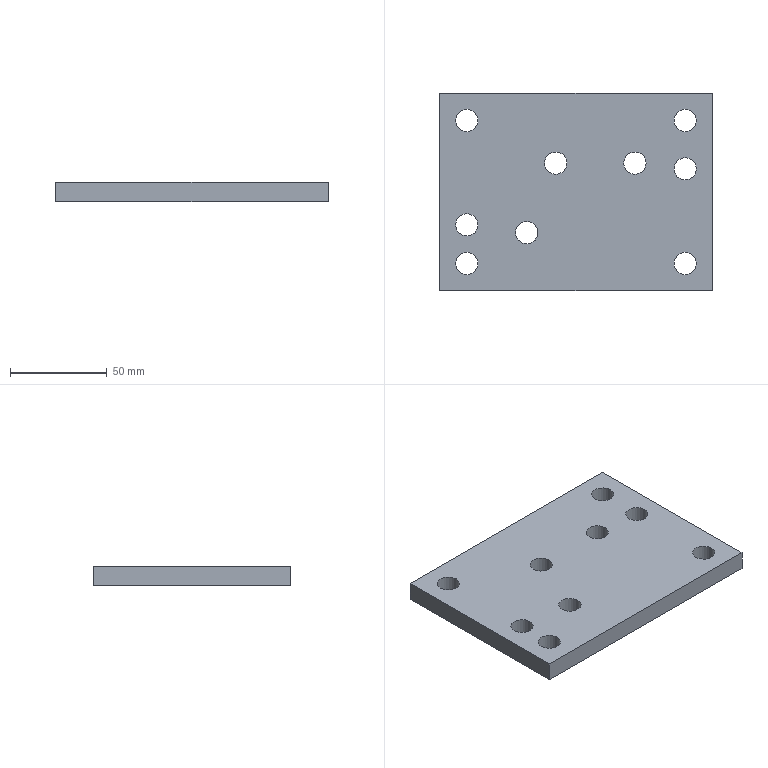Part | NX | features 6 2 | 1 solid | 15 faces | box 141 x 102 x 10 mm | volume 134472 mm3 | cylinder 9 | plane 6 | commonest cylinder face diameters 11.5 x9
STEP:
#1=CARTESIAN_POINT('',(177.279,-375.95,91.));
#2=VERTEX_POINT('',#1);
#3=CARTESIAN_POINT('',(171.529,-375.95,91.));
#4=DIRECTION('',(0.,0.,1.));
#5=DIRECTION('',(1.,0.,0.));
#6=AXIS2_PLACEMENT_3D('',#3,#4,#5);
#7=CIRCLE('',#6,5.75);
#8=EDGE_CURVE('',#2,#2,#7,.T.);
#9=ORIENTED_EDGE('',*,*,#8,.F.);
#10=EDGE_LOOP('',(#9));
#11=FACE_BOUND('',#10,.T.);
#12=CARTESIAN_POINT('',(177.279,-375.95,101.));
#13=VERTEX_POINT('',#12);
#14=CARTESIAN_POINT('',(171.529,-375.95,101.));
#15=DIRECTION('',(0.,0.,1.));
#16=DIRECTION('',(1.,0.,0.));
#17=AXIS2_PLACEMENT_3D('',#14,#15,#16);
#18=CIRCLE('',#17,5.75);
#19=EDGE_CURVE('',#13,#13,#18,.T.);
#20=ORIENTED_EDGE('',*,*,#19,.T.);
#21=EDGE_LOOP('',(#20));
#22=FACE_BOUND('',#21,.T.);
#23=CARTESIAN_POINT('',(171.529,-375.95,91.));
#24=DIRECTION('',(0.,0.,1.));
#25=DIRECTION('',(-1.,0.,0.));
#26=AXIS2_PLACEMENT_3D('',#23,#24,#25);
#27=CYLINDRICAL_SURFACE('',#26,5.75);
#28=ADVANCED_FACE('',(#11,#22),#27,.F.);
#29=CARTESIAN_POINT('',(64.279,-429.95,91.));
#30=VERTEX_POINT('',#29);
#31=CARTESIAN_POINT('',(58.529,-429.95,91.));
#32=DIRECTION('',(0.,0.,1.));
#33=DIRECTION('',(1.,0.,0.));
#34=AXIS2_PLACEMENT_3D('',#31,#32,#33);
#35=CIRCLE('',#34,5.75);
#36=EDGE_CURVE('',#30,#30,#35,.T.);
#37=ORIENTED_EDGE('',*,*,#36,.F.);
#38=EDGE_LOOP('',(#37));
#39=FACE_BOUND('',#38,.T.);
#40=CARTESIAN_POINT('',(64.279,-429.95,101.));
#41=VERTEX_POINT('',#40);
#42=CARTESIAN_POINT('',(58.529,-429.95,101.));
#43=DIRECTION('',(0.,0.,-1.));
#44=DIRECTION('',(1.,0.,0.));
#45=AXIS2_PLACEMENT_3D('',#42,#43,#44);
#46=CIRCLE('',#45,5.75);
#47=EDGE_CURVE('',#41,#41,#46,.T.);
#48=ORIENTED_EDGE('',*,*,#47,.F.);
#49=EDGE_LOOP('',(#48));
#50=FACE_BOUND('',#49,.T.);
#51=CARTESIAN_POINT('',(58.529,-429.95,91.));
#52=DIRECTION('',(0.,0.,1.));
#53=DIRECTION('',(-1.,0.,0.));
#54=AXIS2_PLACEMENT_3D('',#51,#52,#53);
#55=CYLINDRICAL_SURFACE('',#54,5.75);
#56=ADVANCED_FACE('',(#39,#50),#55,.F.);
#57=CARTESIAN_POINT('',(64.279,-375.95,91.));
#58=VERTEX_POINT('',#57);
#59=CARTESIAN_POINT('',(58.529,-375.95,91.));
#60=DIRECTION('',(0.,0.,-1.));
#61=DIRECTION('',(1.,0.,0.));
#62=AXIS2_PLACEMENT_3D('',#59,#60,#61);
#63=CIRCLE('',#62,5.75);
#64=EDGE_CURVE('',#58,#58,#63,.T.);
#65=ORIENTED_EDGE('',*,*,#64,.T.);
#66=EDGE_LOOP('',(#65));
#67=FACE_BOUND('',#66,.T.);
#68=CARTESIAN_POINT('',(64.279,-375.95,101.));
#69=VERTEX_POINT('',#68);
#70=CARTESIAN_POINT('',(58.529,-375.95,101.));
#71=DIRECTION('',(0.,0.,-1.));
#72=DIRECTION('',(1.,0.,0.));
#73=AXIS2_PLACEMENT_3D('',#70,#71,#72);
#74=CIRCLE('',#73,5.75);
#75=EDGE_CURVE('',#69,#69,#74,.T.);
#76=ORIENTED_EDGE('',*,*,#75,.F.);
#77=EDGE_LOOP('',(#76));
#78=FACE_BOUND('',#77,.T.);
#79=CARTESIAN_POINT('',(58.529,-375.95,91.));
#80=DIRECTION('',(0.,0.,1.));
#81=DIRECTION('',(-1.,0.,0.));
#82=AXIS2_PLACEMENT_3D('',#79,#80,#81);
#83=CYLINDRICAL_SURFACE('',#82,5.75);
#84=ADVANCED_FACE('',(#67,#78),#83,.F.);
#85=CARTESIAN_POINT('',(185.529,-463.95,91.));
#86=VERTEX_POINT('',#85);
#87=CARTESIAN_POINT('',(185.529,-463.95,101.));
#88=VERTEX_POINT('',#87);
#89=CARTESIAN_POINT('',(185.529,-463.95,91.));
#90=DIRECTION('',(0.,0.,1.));
#91=VECTOR('',#90,1000.);
#92=LINE('',#89,#91);
#93=EDGE_CURVE('',#86,#88,#92,.T.);
#94=ORIENTED_EDGE('',*,*,#93,.F.);
#95=CARTESIAN_POINT('',(185.529,-361.95,91.));
#96=VERTEX_POINT('',#95);
#97=CARTESIAN_POINT('',(185.529,-411.95,91.));
#98=DIRECTION('',(0.,1.,0.));
#99=VECTOR('',#98,1000.);
#100=LINE('',#97,#99);
#101=EDGE_CURVE('',#86,#96,#100,.T.);
#102=ORIENTED_EDGE('',*,*,#101,.T.);
#103=CARTESIAN_POINT('',(185.529,-361.95,101.));
#104=VERTEX_POINT('',#103);
#105=CARTESIAN_POINT('',(185.529,-361.95,91.));
#106=DIRECTION('',(0.,0.,1.));
#107=VECTOR('',#106,1000.);
#108=LINE('',#105,#107);
#109=EDGE_CURVE('',#96,#104,#108,.T.);
#110=ORIENTED_EDGE('',*,*,#109,.T.);
#111=CARTESIAN_POINT('',(185.529,-411.95,101.));
#112=DIRECTION('',(0.,1.,0.));
#113=VECTOR('',#112,1000.);
#114=LINE('',#111,#113);
#115=EDGE_CURVE('',#88,#104,#114,.T.);
#116=ORIENTED_EDGE('',*,*,#115,.F.);
#117=EDGE_LOOP('',(#94,#102,#110,#116));
#118=FACE_BOUND('',#117,.T.);
#119=CARTESIAN_POINT('',(185.529,-411.95,91.));
#120=DIRECTION('',(-1.,0.,0.));
#121=DIRECTION('',(0.,1.,0.));
#122=AXIS2_PLACEMENT_3D('',#119,#120,#121);
#123=PLANE('',#122);
#124=ADVANCED_FACE('',(#118),#123,.F.);
#125=ORIENTED_EDGE('',*,*,#109,.F.);
#126=CARTESIAN_POINT('',(44.529,-361.95,91.));
#127=VERTEX_POINT('',#126);
#128=CARTESIAN_POINT('',(87.029,-361.95,91.));
#129=DIRECTION('',(-1.,0.,0.));
#130=VECTOR('',#129,1000.);
#131=LINE('',#128,#130);
#132=EDGE_CURVE('',#96,#127,#131,.T.);
#133=ORIENTED_EDGE('',*,*,#132,.T.);
#134=CARTESIAN_POINT('',(44.529,-361.95,101.));
#135=VERTEX_POINT('',#134);
#136=CARTESIAN_POINT('',(44.529,-361.95,91.));
#137=DIRECTION('',(0.,0.,1.));
#138=VECTOR('',#137,1000.);
#139=LINE('',#136,#138);
#140=EDGE_CURVE('',#127,#135,#139,.T.);
#141=ORIENTED_EDGE('',*,*,#140,.T.);
#142=CARTESIAN_POINT('',(87.029,-361.95,101.));
#143=DIRECTION('',(-1.,0.,0.));
#144=VECTOR('',#143,1000.);
#145=LINE('',#142,#144);
#146=EDGE_CURVE('',#104,#135,#145,.T.);
#147=ORIENTED_EDGE('',*,*,#146,.F.);
#148=EDGE_LOOP('',(#125,#133,#141,#147));
#149=FACE_BOUND('',#148,.T.);
#150=CARTESIAN_POINT('',(87.029,-361.95,91.));
#151=DIRECTION('',(0.,-1.,0.));
#152=DIRECTION('',(-1.,0.,0.));
#153=AXIS2_PLACEMENT_3D('',#150,#151,#152);
#154=PLANE('',#153);
#155=ADVANCED_FACE('',(#149),#154,.F.);
#156=ORIENTED_EDGE('',*,*,#140,.F.);
#157=CARTESIAN_POINT('',(44.529,-463.95,91.));
#158=VERTEX_POINT('',#157);
#159=CARTESIAN_POINT('',(44.529,-411.95,91.));
#160=DIRECTION('',(0.,-1.,0.));
#161=VECTOR('',#160,1000.);
#162=LINE('',#159,#161);
#163=EDGE_CURVE('',#127,#158,#162,.T.);
#164=ORIENTED_EDGE('',*,*,#163,.T.);
#165=CARTESIAN_POINT('',(44.529,-463.95,101.));
#166=VERTEX_POINT('',#165);
#167=CARTESIAN_POINT('',(44.529,-463.95,91.));
#168=DIRECTION('',(0.,0.,1.));
#169=VECTOR('',#168,1000.);
#170=LINE('',#167,#169);
#171=EDGE_CURVE('',#158,#166,#170,.T.);
#172=ORIENTED_EDGE('',*,*,#171,.T.);
#173=CARTESIAN_POINT('',(44.529,-411.95,101.));
#174=DIRECTION('',(0.,-1.,0.));
#175=VECTOR('',#174,1000.);
#176=LINE('',#173,#175);
#177=EDGE_CURVE('',#135,#166,#176,.T.);
#178=ORIENTED_EDGE('',*,*,#177,.F.);
#179=EDGE_LOOP('',(#156,#164,#172,#178));
#180=FACE_BOUND('',#179,.T.);
#181=CARTESIAN_POINT('',(44.529,-411.95,91.));
#182=DIRECTION('',(1.,0.,0.));
#183=DIRECTION('',(0.,-1.,0.));
#184=AXIS2_PLACEMENT_3D('',#181,#182,#183);
#185=PLANE('',#184);
#186=ADVANCED_FACE('',(#180),#185,.F.);
#187=ORIENTED_EDGE('',*,*,#171,.F.);
#188=CARTESIAN_POINT('',(87.029,-463.95,91.));
#189=DIRECTION('',(1.,0.,0.));
#190=VECTOR('',#189,1000.);
#191=LINE('',#188,#190);
#192=EDGE_CURVE('',#158,#86,#191,.T.);
#193=ORIENTED_EDGE('',*,*,#192,.T.);
#194=ORIENTED_EDGE('',*,*,#93,.T.);
#195=CARTESIAN_POINT('',(87.029,-463.95,101.));
#196=DIRECTION('',(1.,0.,0.));
#197=VECTOR('',#196,1000.);
#198=LINE('',#195,#197);
#199=EDGE_CURVE('',#166,#88,#198,.T.);
#200=ORIENTED_EDGE('',*,*,#199,.F.);
#201=EDGE_LOOP('',(#187,#193,#194,#200));
#202=FACE_BOUND('',#201,.T.);
#203=CARTESIAN_POINT('',(87.029,-463.95,91.));
#204=DIRECTION('',(0.,1.,0.));
#205=DIRECTION('',(1.,0.,0.));
#206=AXIS2_PLACEMENT_3D('',#203,#204,#205);
#207=PLANE('',#206);
#208=ADVANCED_FACE('',(#202),#207,.F.);
#209=CARTESIAN_POINT('',(177.279,-449.95,91.));
#210=VERTEX_POINT('',#209);
#211=CARTESIAN_POINT('',(171.529,-449.95,91.));
#212=DIRECTION('',(0.,0.,-1.));
#213=DIRECTION('',(1.,0.,0.));
#214=AXIS2_PLACEMENT_3D('',#211,#212,#213);
#215=CIRCLE('',#214,5.75);
#216=EDGE_CURVE('',#210,#210,#215,.T.);
#217=ORIENTED_EDGE('',*,*,#216,.T.);
#218=EDGE_LOOP('',(#217));
#219=FACE_BOUND('',#218,.T.);
#220=CARTESIAN_POINT('',(177.279,-449.95,101.));
#221=VERTEX_POINT('',#220);
#222=CARTESIAN_POINT('',(171.529,-449.95,101.));
#223=DIRECTION('',(0.,0.,-1.));
#224=DIRECTION('',(1.,0.,0.));
#225=AXIS2_PLACEMENT_3D('',#222,#223,#224);
#226=CIRCLE('',#225,5.75);
#227=EDGE_CURVE('',#221,#221,#226,.T.);
#228=ORIENTED_EDGE('',*,*,#227,.F.);
#229=EDGE_LOOP('',(#228));
#230=FACE_BOUND('',#229,.T.);
#231=CARTESIAN_POINT('',(171.529,-449.95,91.));
#232=DIRECTION('',(0.,0.,1.));
#233=DIRECTION('',(-1.,0.,0.));
#234=AXIS2_PLACEMENT_3D('',#231,#232,#233);
#235=CYLINDRICAL_SURFACE('',#234,5.75);
#236=ADVANCED_FACE('',(#219,#230),#235,.F.);
#237=CARTESIAN_POINT('',(177.279,-400.95,91.));
#238=VERTEX_POINT('',#237);
#239=CARTESIAN_POINT('',(171.529,-400.95,91.));
#240=DIRECTION('',(0.,0.,1.));
#241=DIRECTION('',(1.,0.,0.));
#242=AXIS2_PLACEMENT_3D('',#239,#240,#241);
#243=CIRCLE('',#242,5.75);
#244=EDGE_CURVE('',#238,#238,#243,.T.);
#245=ORIENTED_EDGE('',*,*,#244,.F.);
#246=EDGE_LOOP('',(#245));
#247=FACE_BOUND('',#246,.T.);
#248=CARTESIAN_POINT('',(177.279,-400.95,101.));
#249=VERTEX_POINT('',#248);
#250=CARTESIAN_POINT('',(171.529,-400.95,101.));
#251=DIRECTION('',(0.,0.,-1.));
#252=DIRECTION('',(1.,0.,0.));
#253=AXIS2_PLACEMENT_3D('',#250,#251,#252);
#254=CIRCLE('',#253,5.75);
#255=EDGE_CURVE('',#249,#249,#254,.T.);
#256=ORIENTED_EDGE('',*,*,#255,.F.);
#257=EDGE_LOOP('',(#256));
#258=FACE_BOUND('',#257,.T.);
#259=CARTESIAN_POINT('',(171.529,-400.95,91.));
#260=DIRECTION('',(0.,0.,1.));
#261=DIRECTION('',(-1.,0.,0.));
#262=AXIS2_PLACEMENT_3D('',#259,#260,#261);
#263=CYLINDRICAL_SURFACE('',#262,5.75);
#264=ADVANCED_FACE('',(#247,#258),#263,.F.);
#265=CARTESIAN_POINT('',(64.279,-449.95,91.));
#266=VERTEX_POINT('',#265);
#267=CARTESIAN_POINT('',(58.529,-449.95,91.));
#268=DIRECTION('',(0.,0.,1.));
#269=DIRECTION('',(1.,0.,0.));
#270=AXIS2_PLACEMENT_3D('',#267,#268,#269);
#271=CIRCLE('',#270,5.75);
#272=EDGE_CURVE('',#266,#266,#271,.T.);
#273=ORIENTED_EDGE('',*,*,#272,.F.);
#274=EDGE_LOOP('',(#273));
#275=FACE_BOUND('',#274,.T.);
#276=CARTESIAN_POINT('',(64.279,-449.95,101.));
#277=VERTEX_POINT('',#276);
#278=CARTESIAN_POINT('',(58.529,-449.95,101.));
#279=DIRECTION('',(0.,0.,1.));
#280=DIRECTION('',(1.,0.,0.));
#281=AXIS2_PLACEMENT_3D('',#278,#279,#280);
#282=CIRCLE('',#281,5.75);
#283=EDGE_CURVE('',#277,#277,#282,.T.);
#284=ORIENTED_EDGE('',*,*,#283,.T.);
#285=EDGE_LOOP('',(#284));
#286=FACE_BOUND('',#285,.T.);
#287=CARTESIAN_POINT('',(58.529,-449.95,91.));
#288=DIRECTION('',(0.,0.,1.));
#289=DIRECTION('',(-1.,0.,0.));
#290=AXIS2_PLACEMENT_3D('',#287,#288,#289);
#291=CYLINDRICAL_SURFACE('',#290,5.75);
#292=ADVANCED_FACE('',(#275,#286),#291,.F.);
#293=CARTESIAN_POINT('',(95.279,-434.,91.));
#294=VERTEX_POINT('',#293);
#295=CARTESIAN_POINT('',(89.529,-434.,91.));
#296=DIRECTION('',(0.,0.,-1.));
#297=DIRECTION('',(1.,0.,0.));
#298=AXIS2_PLACEMENT_3D('',#295,#296,#297);
#299=CIRCLE('',#298,5.75);
#300=EDGE_CURVE('',#294,#294,#299,.T.);
#301=ORIENTED_EDGE('',*,*,#300,.F.);
#302=EDGE_LOOP('',(#301));
#303=FACE_BOUND('',#302,.T.);
#304=CARTESIAN_POINT('',(110.279,-398.,91.));
#305=VERTEX_POINT('',#304);
#306=CARTESIAN_POINT('',(104.529,-398.,91.));
#307=DIRECTION('',(0.,0.,-1.));
#308=DIRECTION('',(1.,0.,0.));
#309=AXIS2_PLACEMENT_3D('',#306,#307,#308);
#310=CIRCLE('',#309,5.75);
#311=EDGE_CURVE('',#305,#305,#310,.T.);
#312=ORIENTED_EDGE('',*,*,#311,.F.);
#313=EDGE_LOOP('',(#312));
#314=FACE_BOUND('',#313,.T.);
#315=CARTESIAN_POINT('',(151.279,-398.,91.));
#316=VERTEX_POINT('',#315);
#317=CARTESIAN_POINT('',(145.529,-398.,91.));
#318=DIRECTION('',(0.,0.,1.));
#319=DIRECTION('',(1.,0.,0.));
#320=AXIS2_PLACEMENT_3D('',#317,#318,#319);
#321=CIRCLE('',#320,5.75);
#322=EDGE_CURVE('',#316,#316,#321,.T.);
#323=ORIENTED_EDGE('',*,*,#322,.T.);
#324=EDGE_LOOP('',(#323));
#325=FACE_BOUND('',#324,.T.);
#326=ORIENTED_EDGE('',*,*,#8,.T.);
#327=EDGE_LOOP('',(#326));
#328=FACE_BOUND('',#327,.T.);
#329=ORIENTED_EDGE('',*,*,#272,.T.);
#330=EDGE_LOOP('',(#329));
#331=FACE_BOUND('',#330,.T.);
#332=ORIENTED_EDGE('',*,*,#244,.T.);
#333=EDGE_LOOP('',(#332));
#334=FACE_BOUND('',#333,.T.);
#335=ORIENTED_EDGE('',*,*,#216,.F.);
#336=EDGE_LOOP('',(#335));
#337=FACE_BOUND('',#336,.T.);
#338=ORIENTED_EDGE('',*,*,#192,.F.);
#339=ORIENTED_EDGE('',*,*,#163,.F.);
#340=ORIENTED_EDGE('',*,*,#132,.F.);
#341=ORIENTED_EDGE('',*,*,#101,.F.);
#342=EDGE_LOOP('',(#338,#339,#340,#341));
#343=FACE_BOUND('',#342,.T.);
#344=ORIENTED_EDGE('',*,*,#64,.F.);
#345=EDGE_LOOP('',(#344));
#346=FACE_BOUND('',#345,.T.);
#347=ORIENTED_EDGE('',*,*,#36,.T.);
#348=EDGE_LOOP('',(#347));
#349=FACE_BOUND('',#348,.T.);
#350=CARTESIAN_POINT('',(87.029,-411.95,91.));
#351=DIRECTION('',(0.,0.,1.));
#352=DIRECTION('',(-1.,0.,0.));
#353=AXIS2_PLACEMENT_3D('',#350,#351,#352);
#354=PLANE('',#353);
#355=ADVANCED_FACE('',(#303,#314,#325,#328,#331,#334,#337,#343,#346,#349),#354,.F.);
#356=CARTESIAN_POINT('',(95.279,-434.,101.));
#357=VERTEX_POINT('',#356);
#358=CARTESIAN_POINT('',(89.529,-434.,101.));
#359=DIRECTION('',(0.,0.,-1.));
#360=DIRECTION('',(1.,0.,0.));
#361=AXIS2_PLACEMENT_3D('',#358,#359,#360);
#362=CIRCLE('',#361,5.75);
#363=EDGE_CURVE('',#357,#357,#362,.T.);
#364=ORIENTED_EDGE('',*,*,#363,.T.);
#365=EDGE_LOOP('',(#364));
#366=FACE_BOUND('',#365,.T.);
#367=CARTESIAN_POINT('',(110.279,-398.,101.));
#368=VERTEX_POINT('',#367);
#369=CARTESIAN_POINT('',(104.529,-398.,101.));
#370=DIRECTION('',(0.,0.,1.));
#371=DIRECTION('',(1.,0.,0.));
#372=AXIS2_PLACEMENT_3D('',#369,#370,#371);
#373=CIRCLE('',#372,5.75);
#374=EDGE_CURVE('',#368,#368,#373,.T.);
#375=ORIENTED_EDGE('',*,*,#374,.F.);
#376=EDGE_LOOP('',(#375));
#377=FACE_BOUND('',#376,.T.);
#378=CARTESIAN_POINT('',(151.279,-398.,101.));
#379=VERTEX_POINT('',#378);
#380=CARTESIAN_POINT('',(145.529,-398.,101.));
#381=DIRECTION('',(0.,0.,-1.));
#382=DIRECTION('',(1.,0.,0.));
#383=AXIS2_PLACEMENT_3D('',#380,#381,#382);
#384=CIRCLE('',#383,5.75);
#385=EDGE_CURVE('',#379,#379,#384,.T.);
#386=ORIENTED_EDGE('',*,*,#385,.T.);
#387=EDGE_LOOP('',(#386));
#388=FACE_BOUND('',#387,.T.);
#389=ORIENTED_EDGE('',*,*,#19,.F.);
#390=EDGE_LOOP('',(#389));
#391=FACE_BOUND('',#390,.T.);
#392=ORIENTED_EDGE('',*,*,#283,.F.);
#393=EDGE_LOOP('',(#392));
#394=FACE_BOUND('',#393,.T.);
#395=ORIENTED_EDGE('',*,*,#47,.T.);
#396=EDGE_LOOP('',(#395));
#397=FACE_BOUND('',#396,.T.);
#398=ORIENTED_EDGE('',*,*,#75,.T.);
#399=EDGE_LOOP('',(#398));
#400=FACE_BOUND('',#399,.T.);
#401=ORIENTED_EDGE('',*,*,#146,.T.);
#402=ORIENTED_EDGE('',*,*,#177,.T.);
#403=ORIENTED_EDGE('',*,*,#199,.T.);
#404=ORIENTED_EDGE('',*,*,#115,.T.);
#405=EDGE_LOOP('',(#401,#402,#403,#404));
#406=FACE_BOUND('',#405,.T.);
#407=ORIENTED_EDGE('',*,*,#227,.T.);
#408=EDGE_LOOP('',(#407));
#409=FACE_BOUND('',#408,.T.);
#410=ORIENTED_EDGE('',*,*,#255,.T.);
#411=EDGE_LOOP('',(#410));
#412=FACE_BOUND('',#411,.T.);
#413=CARTESIAN_POINT('',(1217.029,-229.95,101.));
#414=DIRECTION('',(0.,0.,1.));
#415=DIRECTION('',(1.,0.,0.));
#416=AXIS2_PLACEMENT_3D('',#413,#414,#415);
#417=PLANE('',#416);
#418=ADVANCED_FACE('',(#366,#377,#388,#391,#394,#397,#400,#406,#409,#412),#417,.T.);
#419=ORIENTED_EDGE('',*,*,#385,.F.);
#420=EDGE_LOOP('',(#419));
#421=FACE_BOUND('',#420,.T.);
#422=ORIENTED_EDGE('',*,*,#322,.F.);
#423=EDGE_LOOP('',(#422));
#424=FACE_BOUND('',#423,.T.);
#425=CARTESIAN_POINT('',(145.529,-398.,-69.));
#426=DIRECTION('',(0.,0.,1.));
#427=DIRECTION('',(-1.,0.,0.));
#428=AXIS2_PLACEMENT_3D('',#425,#426,#427);
#429=CYLINDRICAL_SURFACE('',#428,5.75);
#430=ADVANCED_FACE('',(#421,#424),#429,.F.);
#431=ORIENTED_EDGE('',*,*,#374,.T.);
#432=EDGE_LOOP('',(#431));
#433=FACE_BOUND('',#432,.T.);
#434=ORIENTED_EDGE('',*,*,#311,.T.);
#435=EDGE_LOOP('',(#434));
#436=FACE_BOUND('',#435,.T.);
#437=CARTESIAN_POINT('',(104.529,-398.,-69.));
#438=DIRECTION('',(0.,0.,1.));
#439=DIRECTION('',(-1.,0.,0.));
#440=AXIS2_PLACEMENT_3D('',#437,#438,#439);
#441=CYLINDRICAL_SURFACE('',#440,5.75);
#442=ADVANCED_FACE('',(#433,#436),#441,.F.);
#443=ORIENTED_EDGE('',*,*,#363,.F.);
#444=EDGE_LOOP('',(#443));
#445=FACE_BOUND('',#444,.T.);
#446=ORIENTED_EDGE('',*,*,#300,.T.);
#447=EDGE_LOOP('',(#446));
#448=FACE_BOUND('',#447,.T.);
#449=CARTESIAN_POINT('',(89.529,-434.,-69.));
#450=DIRECTION('',(0.,0.,1.));
#451=DIRECTION('',(-1.,0.,0.));
#452=AXIS2_PLACEMENT_3D('',#449,#450,#451);
#453=CYLINDRICAL_SURFACE('',#452,5.75);
#454=ADVANCED_FACE('',(#445,#448),#453,.F.);
#455=CLOSED_SHELL('',(#28,#56,#84,#124,#155,#186,#208,#236,#264,#292,#355,#418,#430,#442,#454));
#456=MANIFOLD_SOLID_BREP('',#455);
#457=(LENGTH_UNIT()NAMED_UNIT(*)SI_UNIT(.MILLI.,.METRE.));
#458=UNCERTAINTY_MEASURE_WITH_UNIT(LENGTH_MEASURE(0.00001),#457,'','');
#459=(NAMED_UNIT(*)PLANE_ANGLE_UNIT()SI_UNIT($,.RADIAN.));
#460=(NAMED_UNIT(*)SI_UNIT($,.STERADIAN.)SOLID_ANGLE_UNIT());
#461=(GEOMETRIC_REPRESENTATION_CONTEXT(3)GLOBAL_UNCERTAINTY_ASSIGNED_CONTEXT((#458))GLOBAL_UNIT_ASSIGNED_CONTEXT((#457,#459,#460))REPRESENTATION_CONTEXT('',''));
#462=ADVANCED_BREP_SHAPE_REPRESENTATION('',(#456),#461);